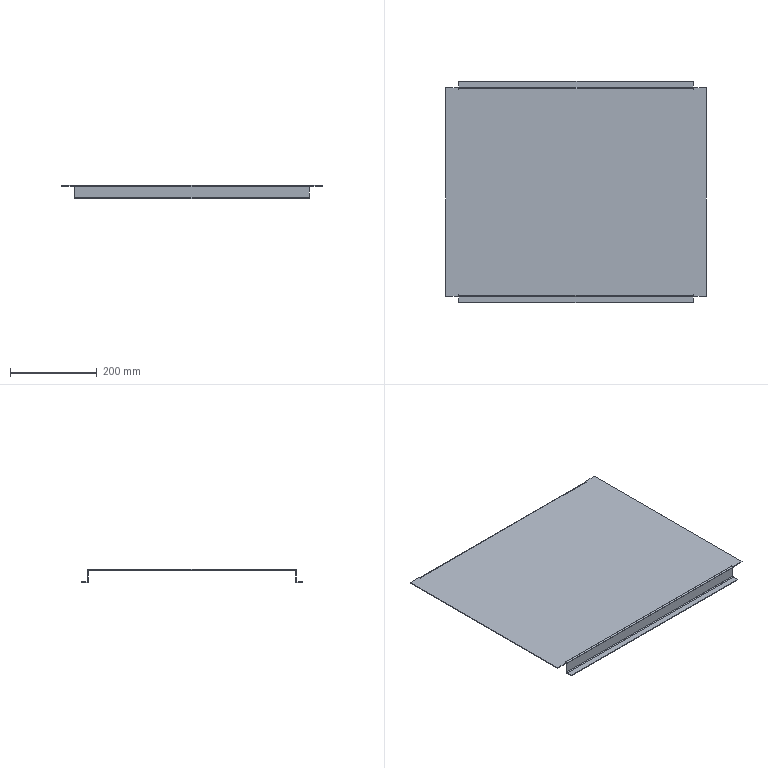Part | SolidWorks | features EdgeFlange 2, FlatPattern 1, SMBaseFlange 1, SheetMetal 1 | 1 solid | 54 faces | box 600 x 510 x 30 mm | volume 499324 mm3 | plane 46 | cylinder 8 | commonest cylinder face diameters 3 x4 6 x4
STEP:
#1=CARTESIAN_POINT('',(-270.,240.,-3.));
#2=VERTEX_POINT('',#1);
#3=CARTESIAN_POINT('',(-270.,240.,-27.));
#4=VERTEX_POINT('',#3);
#5=CARTESIAN_POINT('',(-270.,240.,-1.5));
#6=DIRECTION('',(0.,0.,-1.));
#7=VECTOR('',#6,1000.);
#8=LINE('',#5,#7);
#9=EDGE_CURVE('',#2,#4,#8,.T.);
#10=ORIENTED_EDGE('',*,*,#9,.T.);
#11=CARTESIAN_POINT('',(-270.,238.5,-27.));
#12=VERTEX_POINT('',#11);
#13=CARTESIAN_POINT('',(-270.,240.,-27.));
#14=DIRECTION('',(0.,-1.,0.));
#15=VECTOR('',#14,1000.);
#16=LINE('',#13,#15);
#17=EDGE_CURVE('',#4,#12,#16,.T.);
#18=ORIENTED_EDGE('',*,*,#17,.T.);
#19=CARTESIAN_POINT('',(-270.,238.5,-3.));
#20=VERTEX_POINT('',#19);
#21=CARTESIAN_POINT('',(-270.,238.5,0.));
#22=DIRECTION('',(0.,0.,-1.));
#23=VECTOR('',#22,1000.);
#24=LINE('',#21,#23);
#25=EDGE_CURVE('',#20,#12,#24,.T.);
#26=ORIENTED_EDGE('',*,*,#25,.F.);
#27=CARTESIAN_POINT('',(-270.,240.,-3.));
#28=DIRECTION('',(0.,1.,0.));
#29=VECTOR('',#28,1000.);
#30=LINE('',#27,#29);
#31=EDGE_CURVE('',#20,#2,#30,.T.);
#32=ORIENTED_EDGE('',*,*,#31,.T.);
#33=EDGE_LOOP('',(#10,#18,#26,#32));
#34=FACE_OUTER_BOUND('',#33,.T.);
#35=CARTESIAN_POINT('',(-270.,240.,-1.5));
#36=DIRECTION('',(-1.,0.,0.));
#37=DIRECTION('',(0.,0.,1.));
#38=AXIS2_PLACEMENT_3D('',#35,#36,#37);
#39=PLANE('',#38);
#40=ADVANCED_FACE('',(#34),#39,.T.);
#41=CARTESIAN_POINT('',(270.,240.,-27.));
#42=VERTEX_POINT('',#41);
#43=CARTESIAN_POINT('',(-270.,240.,-27.));
#44=DIRECTION('',(1.,0.,0.));
#45=VECTOR('',#44,1000.);
#46=LINE('',#43,#45);
#47=EDGE_CURVE('',#4,#42,#46,.T.);
#48=ORIENTED_EDGE('',*,*,#47,.F.);
#49=ORIENTED_EDGE('',*,*,#9,.F.);
#50=CARTESIAN_POINT('',(270.,240.,-3.));
#51=VERTEX_POINT('',#50);
#52=CARTESIAN_POINT('',(-270.,240.,-3.));
#53=DIRECTION('',(-1.,0.,0.));
#54=VECTOR('',#53,1000.);
#55=LINE('',#52,#54);
#56=EDGE_CURVE('',#51,#2,#55,.T.);
#57=ORIENTED_EDGE('',*,*,#56,.F.);
#58=CARTESIAN_POINT('',(270.,240.,-30.));
#59=DIRECTION('',(0.,0.,1.));
#60=VECTOR('',#59,1000.);
#61=LINE('',#58,#60);
#62=EDGE_CURVE('',#42,#51,#61,.T.);
#63=ORIENTED_EDGE('',*,*,#62,.F.);
#64=EDGE_LOOP('',(#48,#49,#57,#63));
#65=FACE_OUTER_BOUND('',#64,.T.);
#66=CARTESIAN_POINT('',(0.,240.,0.));
#67=DIRECTION('',(0.,-1.,0.));
#68=DIRECTION('',(0.,0.,-1.));
#69=AXIS2_PLACEMENT_3D('',#66,#67,#68);
#70=PLANE('',#69);
#71=ADVANCED_FACE('',(#65),#70,.F.);
#72=ORIENTED_EDGE('',*,*,#25,.T.);
#73=CARTESIAN_POINT('',(270.,238.5,-27.));
#74=VERTEX_POINT('',#73);
#75=CARTESIAN_POINT('',(-270.,238.5,-27.));
#76=DIRECTION('',(1.,0.,0.));
#77=VECTOR('',#76,1000.);
#78=LINE('',#75,#77);
#79=EDGE_CURVE('',#12,#74,#78,.T.);
#80=ORIENTED_EDGE('',*,*,#79,.T.);
#81=CARTESIAN_POINT('',(270.,238.5,-3.));
#82=VERTEX_POINT('',#81);
#83=CARTESIAN_POINT('',(270.,238.5,0.));
#84=DIRECTION('',(0.,0.,1.));
#85=VECTOR('',#84,1000.);
#86=LINE('',#83,#85);
#87=EDGE_CURVE('',#74,#82,#86,.T.);
#88=ORIENTED_EDGE('',*,*,#87,.T.);
#89=CARTESIAN_POINT('',(-270.,238.5,-3.));
#90=DIRECTION('',(1.,0.,0.));
#91=VECTOR('',#90,1000.);
#92=LINE('',#89,#91);
#93=EDGE_CURVE('',#20,#82,#92,.T.);
#94=ORIENTED_EDGE('',*,*,#93,.F.);
#95=EDGE_LOOP('',(#72,#80,#88,#94));
#96=FACE_OUTER_BOUND('',#95,.T.);
#97=CARTESIAN_POINT('',(0.,238.5,0.));
#98=DIRECTION('',(0.,-1.,0.));
#99=DIRECTION('',(0.,0.,-1.));
#100=AXIS2_PLACEMENT_3D('',#97,#98,#99);
#101=PLANE('',#100);
#102=ADVANCED_FACE('',(#96),#101,.T.);
#103=CARTESIAN_POINT('',(270.,-240.,-3.));
#104=VERTEX_POINT('',#103);
#105=CARTESIAN_POINT('',(270.,-240.,-27.));
#106=VERTEX_POINT('',#105);
#107=CARTESIAN_POINT('',(270.,-240.,-30.));
#108=DIRECTION('',(0.,0.,-1.));
#109=VECTOR('',#108,1000.);
#110=LINE('',#107,#109);
#111=EDGE_CURVE('',#104,#106,#110,.T.);
#112=ORIENTED_EDGE('',*,*,#111,.T.);
#113=CARTESIAN_POINT('',(270.,-238.5,-27.));
#114=VERTEX_POINT('',#113);
#115=CARTESIAN_POINT('',(270.,-240.,-27.));
#116=DIRECTION('',(0.,1.,0.));
#117=VECTOR('',#116,1000.);
#118=LINE('',#115,#117);
#119=EDGE_CURVE('',#106,#114,#118,.T.);
#120=ORIENTED_EDGE('',*,*,#119,.T.);
#121=CARTESIAN_POINT('',(270.,-238.5,-3.));
#122=VERTEX_POINT('',#121);
#123=CARTESIAN_POINT('',(270.,-238.5,0.));
#124=DIRECTION('',(0.,0.,-1.));
#125=VECTOR('',#124,1000.);
#126=LINE('',#123,#125);
#127=EDGE_CURVE('',#122,#114,#126,.T.);
#128=ORIENTED_EDGE('',*,*,#127,.F.);
#129=CARTESIAN_POINT('',(270.,-240.,-3.));
#130=DIRECTION('',(0.,-1.,0.));
#131=VECTOR('',#130,1000.);
#132=LINE('',#129,#131);
#133=EDGE_CURVE('',#122,#104,#132,.T.);
#134=ORIENTED_EDGE('',*,*,#133,.T.);
#135=EDGE_LOOP('',(#112,#120,#128,#134));
#136=FACE_OUTER_BOUND('',#135,.T.);
#137=CARTESIAN_POINT('',(270.,-240.,-30.));
#138=DIRECTION('',(1.,0.,0.));
#139=DIRECTION('',(0.,0.,-1.));
#140=AXIS2_PLACEMENT_3D('',#137,#138,#139);
#141=PLANE('',#140);
#142=ADVANCED_FACE('',(#136),#141,.T.);
#143=CARTESIAN_POINT('',(-270.,-240.,-27.));
#144=VERTEX_POINT('',#143);
#145=CARTESIAN_POINT('',(-270.,-240.,-3.));
#146=VERTEX_POINT('',#145);
#147=CARTESIAN_POINT('',(-270.,-240.,-1.5));
#148=DIRECTION('',(0.,0.,1.));
#149=VECTOR('',#148,1000.);
#150=LINE('',#147,#149);
#151=EDGE_CURVE('',#144,#146,#150,.T.);
#152=ORIENTED_EDGE('',*,*,#151,.F.);
#153=CARTESIAN_POINT('',(270.,-240.,-27.));
#154=DIRECTION('',(-1.,0.,0.));
#155=VECTOR('',#154,1000.);
#156=LINE('',#153,#155);
#157=EDGE_CURVE('',#106,#144,#156,.T.);
#158=ORIENTED_EDGE('',*,*,#157,.F.);
#159=ORIENTED_EDGE('',*,*,#111,.F.);
#160=CARTESIAN_POINT('',(0.,-240.,-3.));
#161=DIRECTION('',(-1.,0.,0.));
#162=VECTOR('',#161,1000.);
#163=LINE('',#160,#162);
#164=EDGE_CURVE('',#104,#146,#163,.T.);
#165=ORIENTED_EDGE('',*,*,#164,.T.);
#166=EDGE_LOOP('',(#152,#158,#159,#165));
#167=FACE_OUTER_BOUND('',#166,.T.);
#168=CARTESIAN_POINT('',(0.,-240.,0.));
#169=DIRECTION('',(0.,-1.,0.));
#170=DIRECTION('',(0.,0.,-1.));
#171=AXIS2_PLACEMENT_3D('',#168,#169,#170);
#172=PLANE('',#171);
#173=ADVANCED_FACE('',(#167),#172,.T.);
#174=CARTESIAN_POINT('',(-270.,-238.5,-27.));
#175=VERTEX_POINT('',#174);
#176=CARTESIAN_POINT('',(270.,-238.5,-27.));
#177=DIRECTION('',(-1.,0.,0.));
#178=VECTOR('',#177,1000.);
#179=LINE('',#176,#178);
#180=EDGE_CURVE('',#114,#175,#179,.T.);
#181=ORIENTED_EDGE('',*,*,#180,.T.);
#182=CARTESIAN_POINT('',(-270.,-238.5,-3.));
#183=VERTEX_POINT('',#182);
#184=CARTESIAN_POINT('',(-270.,-238.5,0.));
#185=DIRECTION('',(0.,0.,1.));
#186=VECTOR('',#185,1000.);
#187=LINE('',#184,#186);
#188=EDGE_CURVE('',#175,#183,#187,.T.);
#189=ORIENTED_EDGE('',*,*,#188,.T.);
#190=CARTESIAN_POINT('',(270.,-238.5,-3.));
#191=DIRECTION('',(-1.,0.,0.));
#192=VECTOR('',#191,1000.);
#193=LINE('',#190,#192);
#194=EDGE_CURVE('',#122,#183,#193,.T.);
#195=ORIENTED_EDGE('',*,*,#194,.F.);
#196=ORIENTED_EDGE('',*,*,#127,.T.);
#197=EDGE_LOOP('',(#181,#189,#195,#196));
#198=FACE_OUTER_BOUND('',#197,.T.);
#199=CARTESIAN_POINT('',(0.,-238.5,0.));
#200=DIRECTION('',(0.,-1.,0.));
#201=DIRECTION('',(0.,0.,-1.));
#202=AXIS2_PLACEMENT_3D('',#199,#200,#201);
#203=PLANE('',#202);
#204=ADVANCED_FACE('',(#198),#203,.F.);
#205=CARTESIAN_POINT('',(270.75,240.,-1.5));
#206=VERTEX_POINT('',#205);
#207=CARTESIAN_POINT('',(270.75,236.25,-1.5));
#208=VERTEX_POINT('',#207);
#209=CARTESIAN_POINT('',(270.75,240.,-1.5));
#210=DIRECTION('',(0.,-1.,0.));
#211=VECTOR('',#210,1000.);
#212=LINE('',#209,#211);
#213=EDGE_CURVE('',#206,#208,#212,.T.);
#214=ORIENTED_EDGE('',*,*,#213,.F.);
#215=CARTESIAN_POINT('',(300.,240.,-1.5));
#216=VERTEX_POINT('',#215);
#217=CARTESIAN_POINT('',(-300.,240.,-1.5));
#218=DIRECTION('',(-1.,0.,0.));
#219=VECTOR('',#218,1000.);
#220=LINE('',#217,#219);
#221=EDGE_CURVE('',#216,#206,#220,.T.);
#222=ORIENTED_EDGE('',*,*,#221,.F.);
#223=CARTESIAN_POINT('',(300.,-240.,-1.5));
#224=VERTEX_POINT('',#223);
#225=CARTESIAN_POINT('',(300.,240.,-1.5));
#226=DIRECTION('',(0.,1.,0.));
#227=VECTOR('',#226,1000.);
#228=LINE('',#225,#227);
#229=EDGE_CURVE('',#224,#216,#228,.T.);
#230=ORIENTED_EDGE('',*,*,#229,.F.);
#231=CARTESIAN_POINT('',(270.75,-240.,-1.5));
#232=VERTEX_POINT('',#231);
#233=CARTESIAN_POINT('',(-300.,-240.,-1.5));
#234=DIRECTION('',(1.,0.,0.));
#235=VECTOR('',#234,1000.);
#236=LINE('',#233,#235);
#237=EDGE_CURVE('',#232,#224,#236,.T.);
#238=ORIENTED_EDGE('',*,*,#237,.F.);
#239=CARTESIAN_POINT('',(270.75,-236.25,-1.5));
#240=VERTEX_POINT('',#239);
#241=CARTESIAN_POINT('',(270.75,-236.25,-1.5));
#242=DIRECTION('',(0.,-1.,0.));
#243=VECTOR('',#242,1000.);
#244=LINE('',#241,#243);
#245=EDGE_CURVE('',#240,#232,#244,.T.);
#246=ORIENTED_EDGE('',*,*,#245,.F.);
#247=CARTESIAN_POINT('',(270.,-236.25,-1.5));
#248=VERTEX_POINT('',#247);
#249=CARTESIAN_POINT('',(270.,-236.25,-1.5));
#250=DIRECTION('',(1.,0.,0.));
#251=VECTOR('',#250,1000.);
#252=LINE('',#249,#251);
#253=EDGE_CURVE('',#248,#240,#252,.T.);
#254=ORIENTED_EDGE('',*,*,#253,.F.);
#255=CARTESIAN_POINT('',(270.,-237.,-1.5));
#256=VERTEX_POINT('',#255);
#257=CARTESIAN_POINT('',(270.,-237.,-1.5));
#258=DIRECTION('',(0.,1.,0.));
#259=VECTOR('',#258,1000.);
#260=LINE('',#257,#259);
#261=EDGE_CURVE('',#256,#248,#260,.T.);
#262=ORIENTED_EDGE('',*,*,#261,.F.);
#263=CARTESIAN_POINT('',(-270.,-237.,-1.5));
#264=VERTEX_POINT('',#263);
#265=CARTESIAN_POINT('',(-270.,-237.,-1.5));
#266=DIRECTION('',(1.,0.,0.));
#267=VECTOR('',#266,1000.);
#268=LINE('',#265,#267);
#269=EDGE_CURVE('',#264,#256,#268,.T.);
#270=ORIENTED_EDGE('',*,*,#269,.F.);
#271=CARTESIAN_POINT('',(-270.,-236.25,-1.5));
#272=VERTEX_POINT('',#271);
#273=CARTESIAN_POINT('',(-270.,-236.25,-1.5));
#274=DIRECTION('',(0.,-1.,0.));
#275=VECTOR('',#274,1000.);
#276=LINE('',#273,#275);
#277=EDGE_CURVE('',#272,#264,#276,.T.);
#278=ORIENTED_EDGE('',*,*,#277,.F.);
#279=CARTESIAN_POINT('',(-270.75,-236.25,-1.5));
#280=VERTEX_POINT('',#279);
#281=CARTESIAN_POINT('',(-270.75,-236.25,-1.5));
#282=DIRECTION('',(1.,0.,0.));
#283=VECTOR('',#282,1000.);
#284=LINE('',#281,#283);
#285=EDGE_CURVE('',#280,#272,#284,.T.);
#286=ORIENTED_EDGE('',*,*,#285,.F.);
#287=CARTESIAN_POINT('',(-270.75,-240.,-1.5));
#288=VERTEX_POINT('',#287);
#289=CARTESIAN_POINT('',(-270.75,-240.,-1.5));
#290=DIRECTION('',(0.,1.,0.));
#291=VECTOR('',#290,1000.);
#292=LINE('',#289,#291);
#293=EDGE_CURVE('',#288,#280,#292,.T.);
#294=ORIENTED_EDGE('',*,*,#293,.F.);
#295=CARTESIAN_POINT('',(-300.,-240.,-1.5));
#296=VERTEX_POINT('',#295);
#297=CARTESIAN_POINT('',(-300.,-240.,-1.5));
#298=DIRECTION('',(1.,0.,0.));
#299=VECTOR('',#298,1000.);
#300=LINE('',#297,#299);
#301=EDGE_CURVE('',#296,#288,#300,.T.);
#302=ORIENTED_EDGE('',*,*,#301,.F.);
#303=CARTESIAN_POINT('',(-300.,240.,-1.5));
#304=VERTEX_POINT('',#303);
#305=CARTESIAN_POINT('',(-300.,240.,-1.5));
#306=DIRECTION('',(0.,-1.,0.));
#307=VECTOR('',#306,1000.);
#308=LINE('',#305,#307);
#309=EDGE_CURVE('',#304,#296,#308,.T.);
#310=ORIENTED_EDGE('',*,*,#309,.F.);
#311=CARTESIAN_POINT('',(-270.75,240.,-1.5));
#312=VERTEX_POINT('',#311);
#313=CARTESIAN_POINT('',(-300.,240.,-1.5));
#314=DIRECTION('',(-1.,0.,0.));
#315=VECTOR('',#314,1000.);
#316=LINE('',#313,#315);
#317=EDGE_CURVE('',#312,#304,#316,.T.);
#318=ORIENTED_EDGE('',*,*,#317,.F.);
#319=CARTESIAN_POINT('',(-270.75,236.25,-1.5));
#320=VERTEX_POINT('',#319);
#321=CARTESIAN_POINT('',(-270.75,236.25,-1.5));
#322=DIRECTION('',(0.,1.,0.));
#323=VECTOR('',#322,1000.);
#324=LINE('',#321,#323);
#325=EDGE_CURVE('',#320,#312,#324,.T.);
#326=ORIENTED_EDGE('',*,*,#325,.F.);
#327=CARTESIAN_POINT('',(-270.,236.25,-1.5));
#328=VERTEX_POINT('',#327);
#329=CARTESIAN_POINT('',(-270.,236.25,-1.5));
#330=DIRECTION('',(-1.,0.,0.));
#331=VECTOR('',#330,1000.);
#332=LINE('',#329,#331);
#333=EDGE_CURVE('',#328,#320,#332,.T.);
#334=ORIENTED_EDGE('',*,*,#333,.F.);
#335=CARTESIAN_POINT('',(-270.,237.,-1.5));
#336=VERTEX_POINT('',#335);
#337=CARTESIAN_POINT('',(-270.,237.,-1.5));
#338=DIRECTION('',(0.,-1.,0.));
#339=VECTOR('',#338,1000.);
#340=LINE('',#337,#339);
#341=EDGE_CURVE('',#336,#328,#340,.T.);
#342=ORIENTED_EDGE('',*,*,#341,.F.);
#343=CARTESIAN_POINT('',(270.,237.,-1.5));
#344=VERTEX_POINT('',#343);
#345=CARTESIAN_POINT('',(270.,237.,-1.5));
#346=DIRECTION('',(-1.,0.,0.));
#347=VECTOR('',#346,1000.);
#348=LINE('',#345,#347);
#349=EDGE_CURVE('',#344,#336,#348,.T.);
#350=ORIENTED_EDGE('',*,*,#349,.F.);
#351=CARTESIAN_POINT('',(270.,236.25,-1.5));
#352=VERTEX_POINT('',#351);
#353=CARTESIAN_POINT('',(270.,236.25,-1.5));
#354=DIRECTION('',(0.,1.,0.));
#355=VECTOR('',#354,1000.);
#356=LINE('',#353,#355);
#357=EDGE_CURVE('',#352,#344,#356,.T.);
#358=ORIENTED_EDGE('',*,*,#357,.F.);
#359=CARTESIAN_POINT('',(270.75,236.25,-1.5));
#360=DIRECTION('',(-1.,0.,0.));
#361=VECTOR('',#360,1000.);
#362=LINE('',#359,#361);
#363=EDGE_CURVE('',#208,#352,#362,.T.);
#364=ORIENTED_EDGE('',*,*,#363,.F.);
#365=EDGE_LOOP('',(#214,#222,#230,#238,#246,#254,#262,#270,#278,#286,#294,#302,#310,#318,#326,#334,#342,#350,#358,#364));
#366=FACE_OUTER_BOUND('',#365,.T.);
#367=CARTESIAN_POINT('',(0.,0.,-1.5));
#368=DIRECTION('',(0.,0.,1.));
#369=DIRECTION('',(1.,0.,0.));
#370=AXIS2_PLACEMENT_3D('',#367,#368,#369);
#371=PLANE('',#370);
#372=ADVANCED_FACE('',(#366),#371,.F.);
#373=CARTESIAN_POINT('',(300.,240.,0.));
#374=VERTEX_POINT('',#373);
#375=CARTESIAN_POINT('',(270.75,240.,0.));
#376=VERTEX_POINT('',#375);
#377=CARTESIAN_POINT('',(-300.,240.,0.));
#378=DIRECTION('',(-1.,0.,0.));
#379=VECTOR('',#378,1000.);
#380=LINE('',#377,#379);
#381=EDGE_CURVE('',#374,#376,#380,.T.);
#382=ORIENTED_EDGE('',*,*,#381,.T.);
#383=CARTESIAN_POINT('',(270.75,236.25,0.));
#384=VERTEX_POINT('',#383);
#385=CARTESIAN_POINT('',(270.75,0.,0.));
#386=DIRECTION('',(0.,-1.,0.));
#387=VECTOR('',#386,1000.);
#388=LINE('',#385,#387);
#389=EDGE_CURVE('',#376,#384,#388,.T.);
#390=ORIENTED_EDGE('',*,*,#389,.T.);
#391=CARTESIAN_POINT('',(270.,236.25,0.));
#392=VERTEX_POINT('',#391);
#393=CARTESIAN_POINT('',(0.,236.25,0.));
#394=DIRECTION('',(-1.,0.,0.));
#395=VECTOR('',#394,1000.);
#396=LINE('',#393,#395);
#397=EDGE_CURVE('',#384,#392,#396,.T.);
#398=ORIENTED_EDGE('',*,*,#397,.T.);
#399=CARTESIAN_POINT('',(270.,237.,0.));
#400=VERTEX_POINT('',#399);
#401=CARTESIAN_POINT('',(270.,0.,0.));
#402=DIRECTION('',(0.,1.,0.));
#403=VECTOR('',#402,1000.);
#404=LINE('',#401,#403);
#405=EDGE_CURVE('',#392,#400,#404,.T.);
#406=ORIENTED_EDGE('',*,*,#405,.T.);
#407=CARTESIAN_POINT('',(-270.,237.,0.));
#408=VERTEX_POINT('',#407);
#409=CARTESIAN_POINT('',(270.,237.,0.));
#410=DIRECTION('',(-1.,0.,0.));
#411=VECTOR('',#410,1000.);
#412=LINE('',#409,#411);
#413=EDGE_CURVE('',#400,#408,#412,.T.);
#414=ORIENTED_EDGE('',*,*,#413,.T.);
#415=CARTESIAN_POINT('',(-270.,236.25,0.));
#416=VERTEX_POINT('',#415);
#417=CARTESIAN_POINT('',(-270.,0.,0.));
#418=DIRECTION('',(0.,-1.,0.));
#419=VECTOR('',#418,1000.);
#420=LINE('',#417,#419);
#421=EDGE_CURVE('',#408,#416,#420,.T.);
#422=ORIENTED_EDGE('',*,*,#421,.T.);
#423=CARTESIAN_POINT('',(-270.75,236.25,0.));
#424=VERTEX_POINT('',#423);
#425=CARTESIAN_POINT('',(0.,236.25,0.));
#426=DIRECTION('',(-1.,0.,0.));
#427=VECTOR('',#426,1000.);
#428=LINE('',#425,#427);
#429=EDGE_CURVE('',#416,#424,#428,.T.);
#430=ORIENTED_EDGE('',*,*,#429,.T.);
#431=CARTESIAN_POINT('',(-270.75,240.,0.));
#432=VERTEX_POINT('',#431);
#433=CARTESIAN_POINT('',(-270.75,0.,0.));
#434=DIRECTION('',(0.,1.,0.));
#435=VECTOR('',#434,1000.);
#436=LINE('',#433,#435);
#437=EDGE_CURVE('',#424,#432,#436,.T.);
#438=ORIENTED_EDGE('',*,*,#437,.T.);
#439=CARTESIAN_POINT('',(-300.,240.,0.));
#440=VERTEX_POINT('',#439);
#441=CARTESIAN_POINT('',(-300.,240.,0.));
#442=DIRECTION('',(-1.,0.,0.));
#443=VECTOR('',#442,1000.);
#444=LINE('',#441,#443);
#445=EDGE_CURVE('',#432,#440,#444,.T.);
#446=ORIENTED_EDGE('',*,*,#445,.T.);
#447=CARTESIAN_POINT('',(-300.,-240.,0.));
#448=VERTEX_POINT('',#447);
#449=CARTESIAN_POINT('',(-300.,240.,0.));
#450=DIRECTION('',(0.,-1.,0.));
#451=VECTOR('',#450,1000.);
#452=LINE('',#449,#451);
#453=EDGE_CURVE('',#440,#448,#452,.T.);
#454=ORIENTED_EDGE('',*,*,#453,.T.);
#455=CARTESIAN_POINT('',(-270.75,-240.,0.));
#456=VERTEX_POINT('',#455);
#457=CARTESIAN_POINT('',(-300.,-240.,0.));
#458=DIRECTION('',(1.,0.,0.));
#459=VECTOR('',#458,1000.);
#460=LINE('',#457,#459);
#461=EDGE_CURVE('',#448,#456,#460,.T.);
#462=ORIENTED_EDGE('',*,*,#461,.T.);
#463=CARTESIAN_POINT('',(-270.75,-236.25,0.));
#464=VERTEX_POINT('',#463);
#465=CARTESIAN_POINT('',(-270.75,0.,0.));
#466=DIRECTION('',(0.,1.,0.));
#467=VECTOR('',#466,1000.);
#468=LINE('',#465,#467);
#469=EDGE_CURVE('',#456,#464,#468,.T.);
#470=ORIENTED_EDGE('',*,*,#469,.T.);
#471=CARTESIAN_POINT('',(-270.,-236.25,0.));
#472=VERTEX_POINT('',#471);
#473=CARTESIAN_POINT('',(0.,-236.25,0.));
#474=DIRECTION('',(1.,0.,0.));
#475=VECTOR('',#474,1000.);
#476=LINE('',#473,#475);
#477=EDGE_CURVE('',#464,#472,#476,.T.);
#478=ORIENTED_EDGE('',*,*,#477,.T.);
#479=CARTESIAN_POINT('',(-270.,-237.,0.));
#480=VERTEX_POINT('',#479);
#481=CARTESIAN_POINT('',(-270.,0.,0.));
#482=DIRECTION('',(0.,-1.,0.));
#483=VECTOR('',#482,1000.);
#484=LINE('',#481,#483);
#485=EDGE_CURVE('',#472,#480,#484,.T.);
#486=ORIENTED_EDGE('',*,*,#485,.T.);
#487=CARTESIAN_POINT('',(270.,-237.,0.));
#488=VERTEX_POINT('',#487);
#489=CARTESIAN_POINT('',(-270.,-237.,0.));
#490=DIRECTION('',(1.,0.,0.));
#491=VECTOR('',#490,1000.);
#492=LINE('',#489,#491);
#493=EDGE_CURVE('',#480,#488,#492,.T.);
#494=ORIENTED_EDGE('',*,*,#493,.T.);
#495=CARTESIAN_POINT('',(270.,-236.25,0.));
#496=VERTEX_POINT('',#495);
#497=CARTESIAN_POINT('',(270.,0.,0.));
#498=DIRECTION('',(0.,1.,0.));
#499=VECTOR('',#498,1000.);
#500=LINE('',#497,#499);
#501=EDGE_CURVE('',#488,#496,#500,.T.);
#502=ORIENTED_EDGE('',*,*,#501,.T.);
#503=CARTESIAN_POINT('',(270.75,-236.25,0.));
#504=VERTEX_POINT('',#503);
#505=CARTESIAN_POINT('',(0.,-236.25,0.));
#506=DIRECTION('',(1.,0.,0.));
#507=VECTOR('',#506,1000.);
#508=LINE('',#505,#507);
#509=EDGE_CURVE('',#496,#504,#508,.T.);
#510=ORIENTED_EDGE('',*,*,#509,.T.);
#511=CARTESIAN_POINT('',(270.75,-240.,0.));
#512=VERTEX_POINT('',#511);
#513=CARTESIAN_POINT('',(270.75,0.,0.));
#514=DIRECTION('',(0.,-1.,0.));
#515=VECTOR('',#514,1000.);
#516=LINE('',#513,#515);
#517=EDGE_CURVE('',#504,#512,#516,.T.);
#518=ORIENTED_EDGE('',*,*,#517,.T.);
#519=CARTESIAN_POINT('',(300.,-240.,0.));
#520=VERTEX_POINT('',#519);
#521=CARTESIAN_POINT('',(-300.,-240.,0.));
#522=DIRECTION('',(1.,0.,0.));
#523=VECTOR('',#522,1000.);
#524=LINE('',#521,#523);
#525=EDGE_CURVE('',#512,#520,#524,.T.);
#526=ORIENTED_EDGE('',*,*,#525,.T.);
#527=CARTESIAN_POINT('',(300.,240.,0.));
#528=DIRECTION('',(0.,1.,0.));
#529=VECTOR('',#528,1000.);
#530=LINE('',#527,#529);
#531=EDGE_CURVE('',#520,#374,#530,.T.);
#532=ORIENTED_EDGE('',*,*,#531,.T.);
#533=EDGE_LOOP('',(#382,#390,#398,#406,#414,#422,#430,#438,#446,#454,#462,#470,#478,#486,#494,#502,#510,#518,#526,#532));
#534=FACE_OUTER_BOUND('',#533,.T.);
#535=CARTESIAN_POINT('',(0.,0.,0.));
#536=DIRECTION('',(0.,0.,1.));
#537=DIRECTION('',(1.,0.,0.));
#538=AXIS2_PLACEMENT_3D('',#535,#536,#537);
#539=PLANE('',#538);
#540=ADVANCED_FACE('',(#534),#539,.T.);
#541=ORIENTED_EDGE('',*,*,#221,.T.);
#542=CARTESIAN_POINT('',(270.75,240.,-1.5));
#543=DIRECTION('',(0.,0.,1.));
#544=VECTOR('',#543,1000.);
#545=LINE('',#542,#544);
#546=EDGE_CURVE('',#206,#376,#545,.T.);
#547=ORIENTED_EDGE('',*,*,#546,.T.);
#548=ORIENTED_EDGE('',*,*,#381,.F.);
#549=CARTESIAN_POINT('',(300.,240.,-1.5));
#550=DIRECTION('',(0.,0.,1.));
#551=VECTOR('',#550,1000.);
#552=LINE('',#549,#551);
#553=EDGE_CURVE('',#216,#374,#552,.T.);
#554=ORIENTED_EDGE('',*,*,#553,.F.);
#555=EDGE_LOOP('',(#541,#547,#548,#554));
#556=FACE_OUTER_BOUND('',#555,.T.);
#557=CARTESIAN_POINT('',(-300.,240.,-1.5));
#558=DIRECTION('',(0.,1.,0.));
#559=DIRECTION('',(0.,0.,1.));
#560=AXIS2_PLACEMENT_3D('',#557,#558,#559);
#561=PLANE('',#560);
#562=ADVANCED_FACE('',(#556),#561,.T.);
#563=ORIENTED_EDGE('',*,*,#445,.F.);
#564=CARTESIAN_POINT('',(-270.75,240.,-1.5));
#565=DIRECTION('',(0.,0.,1.));
#566=VECTOR('',#565,1000.);
#567=LINE('',#564,#566);
#568=EDGE_CURVE('',#312,#432,#567,.T.);
#569=ORIENTED_EDGE('',*,*,#568,.F.);
#570=ORIENTED_EDGE('',*,*,#317,.T.);
#571=CARTESIAN_POINT('',(-300.,240.,-1.5));
#572=DIRECTION('',(0.,0.,1.));
#573=VECTOR('',#572,1000.);
#574=LINE('',#571,#573);
#575=EDGE_CURVE('',#304,#440,#574,.T.);
#576=ORIENTED_EDGE('',*,*,#575,.T.);
#577=EDGE_LOOP('',(#563,#569,#570,#576));
#578=FACE_OUTER_BOUND('',#577,.T.);
#579=CARTESIAN_POINT('',(-300.,240.,-1.5));
#580=DIRECTION('',(0.,1.,0.));
#581=DIRECTION('',(0.,0.,1.));
#582=AXIS2_PLACEMENT_3D('',#579,#580,#581);
#583=PLANE('',#582);
#584=ADVANCED_FACE('',(#578),#583,.T.);
#585=ORIENTED_EDGE('',*,*,#301,.T.);
#586=CARTESIAN_POINT('',(-270.75,-240.,-1.5));
#587=DIRECTION('',(0.,0.,1.));
#588=VECTOR('',#587,1000.);
#589=LINE('',#586,#588);
#590=EDGE_CURVE('',#288,#456,#589,.T.);
#591=ORIENTED_EDGE('',*,*,#590,.T.);
#592=ORIENTED_EDGE('',*,*,#461,.F.);
#593=CARTESIAN_POINT('',(-300.,-240.,-1.5));
#594=DIRECTION('',(0.,0.,1.));
#595=VECTOR('',#594,1000.);
#596=LINE('',#593,#595);
#597=EDGE_CURVE('',#296,#448,#596,.T.);
#598=ORIENTED_EDGE('',*,*,#597,.F.);
#599=EDGE_LOOP('',(#585,#591,#592,#598));
#600=FACE_OUTER_BOUND('',#599,.T.);
#601=CARTESIAN_POINT('',(-300.,-240.,-1.5));
#602=DIRECTION('',(0.,-1.,0.));
#603=DIRECTION('',(0.,0.,-1.));
#604=AXIS2_PLACEMENT_3D('',#601,#602,#603);
#605=PLANE('',#604);
#606=ADVANCED_FACE('',(#600),#605,.T.);
#607=ORIENTED_EDGE('',*,*,#525,.F.);
#608=CARTESIAN_POINT('',(270.75,-240.,-1.5));
#609=DIRECTION('',(0.,0.,1.));
#610=VECTOR('',#609,1000.);
#611=LINE('',#608,#610);
#612=EDGE_CURVE('',#232,#512,#611,.T.);
#613=ORIENTED_EDGE('',*,*,#612,.F.);
#614=ORIENTED_EDGE('',*,*,#237,.T.);
#615=CARTESIAN_POINT('',(300.,-240.,-1.5));
#616=DIRECTION('',(0.,0.,1.));
#617=VECTOR('',#616,1000.);
#618=LINE('',#615,#617);
#619=EDGE_CURVE('',#224,#520,#618,.T.);
#620=ORIENTED_EDGE('',*,*,#619,.T.);
#621=EDGE_LOOP('',(#607,#613,#614,#620));
#622=FACE_OUTER_BOUND('',#621,.T.);
#623=CARTESIAN_POINT('',(-300.,-240.,-1.5));
#624=DIRECTION('',(0.,-1.,0.));
#625=DIRECTION('',(0.,0.,-1.));
#626=AXIS2_PLACEMENT_3D('',#623,#624,#625);
#627=PLANE('',#626);
#628=ADVANCED_FACE('',(#622),#627,.T.);
#629=ORIENTED_EDGE('',*,*,#531,.F.);
#630=ORIENTED_EDGE('',*,*,#619,.F.);
#631=ORIENTED_EDGE('',*,*,#229,.T.);
#632=ORIENTED_EDGE('',*,*,#553,.T.);
#633=EDGE_LOOP('',(#629,#630,#631,#632));
#634=FACE_OUTER_BOUND('',#633,.T.);
#635=CARTESIAN_POINT('',(300.,240.,-1.5));
#636=DIRECTION('',(1.,0.,0.));
#637=DIRECTION('',(0.,1.,0.));
#638=AXIS2_PLACEMENT_3D('',#635,#636,#637);
#639=PLANE('',#638);
#640=ADVANCED_FACE('',(#634),#639,.T.);
#641=ORIENTED_EDGE('',*,*,#453,.F.);
#642=ORIENTED_EDGE('',*,*,#575,.F.);
#643=ORIENTED_EDGE('',*,*,#309,.T.);
#644=ORIENTED_EDGE('',*,*,#597,.T.);
#645=EDGE_LOOP('',(#641,#642,#643,#644));
#646=FACE_OUTER_BOUND('',#645,.T.);
#647=CARTESIAN_POINT('',(-300.,240.,-1.5));
#648=DIRECTION('',(-1.,0.,0.));
#649=DIRECTION('',(0.,-1.,0.));
#650=AXIS2_PLACEMENT_3D('',#647,#648,#649);
#651=PLANE('',#650);
#652=ADVANCED_FACE('',(#646),#651,.T.);
#653=ORIENTED_EDGE('',*,*,#469,.F.);
#654=ORIENTED_EDGE('',*,*,#590,.F.);
#655=ORIENTED_EDGE('',*,*,#293,.T.);
#656=CARTESIAN_POINT('',(-270.75,-236.25,-1.5));
#657=DIRECTION('',(0.,0.,1.));
#658=VECTOR('',#657,1000.);
#659=LINE('',#656,#658);
#660=EDGE_CURVE('',#280,#464,#659,.T.);
#661=ORIENTED_EDGE('',*,*,#660,.T.);
#662=EDGE_LOOP('',(#653,#654,#655,#661));
#663=FACE_OUTER_BOUND('',#662,.T.);
#664=CARTESIAN_POINT('',(-270.75,-240.,-1.5));
#665=DIRECTION('',(1.,0.,0.));
#666=DIRECTION('',(0.,0.,-1.));
#667=AXIS2_PLACEMENT_3D('',#664,#665,#666);
#668=PLANE('',#667);
#669=ADVANCED_FACE('',(#663),#668,.T.);
#670=ORIENTED_EDGE('',*,*,#477,.F.);
#671=ORIENTED_EDGE('',*,*,#660,.F.);
#672=ORIENTED_EDGE('',*,*,#285,.T.);
#673=CARTESIAN_POINT('',(-270.,-236.25,-1.5));
#674=DIRECTION('',(0.,0.,1.));
#675=VECTOR('',#674,1000.);
#676=LINE('',#673,#675);
#677=EDGE_CURVE('',#272,#472,#676,.T.);
#678=ORIENTED_EDGE('',*,*,#677,.T.);
#679=EDGE_LOOP('',(#670,#671,#672,#678));
#680=FACE_OUTER_BOUND('',#679,.T.);
#681=CARTESIAN_POINT('',(-270.75,-236.25,-1.5));
#682=DIRECTION('',(0.,-1.,0.));
#683=DIRECTION('',(0.,0.,-1.));
#684=AXIS2_PLACEMENT_3D('',#681,#682,#683);
#685=PLANE('',#684);
#686=ADVANCED_FACE('',(#680),#685,.T.);
#687=ORIENTED_EDGE('',*,*,#485,.F.);
#688=ORIENTED_EDGE('',*,*,#677,.F.);
#689=ORIENTED_EDGE('',*,*,#277,.T.);
#690=CARTESIAN_POINT('',(-270.,-237.,-1.5));
#691=DIRECTION('',(0.,0.,1.));
#692=VECTOR('',#691,1000.);
#693=LINE('',#690,#692);
#694=EDGE_CURVE('',#264,#480,#693,.T.);
#695=ORIENTED_EDGE('',*,*,#694,.T.);
#696=EDGE_LOOP('',(#687,#688,#689,#695));
#697=FACE_OUTER_BOUND('',#696,.T.);
#698=CARTESIAN_POINT('',(-270.,-236.25,-1.5));
#699=DIRECTION('',(-1.,0.,0.));
#700=DIRECTION('',(0.,0.,1.));
#701=AXIS2_PLACEMENT_3D('',#698,#699,#700);
#702=PLANE('',#701);
#703=ADVANCED_FACE('',(#697),#702,.T.);
#704=ORIENTED_EDGE('',*,*,#501,.F.);
#705=CARTESIAN_POINT('',(270.,-237.,-1.5));
#706=DIRECTION('',(0.,0.,1.));
#707=VECTOR('',#706,1000.);
#708=LINE('',#705,#707);
#709=EDGE_CURVE('',#256,#488,#708,.T.);
#710=ORIENTED_EDGE('',*,*,#709,.F.);
#711=ORIENTED_EDGE('',*,*,#261,.T.);
#712=CARTESIAN_POINT('',(270.,-236.25,-1.5));
#713=DIRECTION('',(0.,0.,1.));
#714=VECTOR('',#713,1000.);
#715=LINE('',#712,#714);
#716=EDGE_CURVE('',#248,#496,#715,.T.);
#717=ORIENTED_EDGE('',*,*,#716,.T.);
#718=EDGE_LOOP('',(#704,#710,#711,#717));
#719=FACE_OUTER_BOUND('',#718,.T.);
#720=CARTESIAN_POINT('',(270.,-237.,-1.5));
#721=DIRECTION('',(1.,0.,0.));
#722=DIRECTION('',(0.,0.,-1.));
#723=AXIS2_PLACEMENT_3D('',#720,#721,#722);
#724=PLANE('',#723);
#725=ADVANCED_FACE('',(#719),#724,.T.);
#726=ORIENTED_EDGE('',*,*,#509,.F.);
#727=ORIENTED_EDGE('',*,*,#716,.F.);
#728=ORIENTED_EDGE('',*,*,#253,.T.);
#729=CARTESIAN_POINT('',(270.75,-236.25,-1.5));
#730=DIRECTION('',(0.,0.,1.));
#731=VECTOR('',#730,1000.);
#732=LINE('',#729,#731);
#733=EDGE_CURVE('',#240,#504,#732,.T.);
#734=ORIENTED_EDGE('',*,*,#733,.T.);
#735=EDGE_LOOP('',(#726,#727,#728,#734));
#736=FACE_OUTER_BOUND('',#735,.T.);
#737=CARTESIAN_POINT('',(270.,-236.25,-1.5));
#738=DIRECTION('',(0.,-1.,0.));
#739=DIRECTION('',(0.,0.,-1.));
#740=AXIS2_PLACEMENT_3D('',#737,#738,#739);
#741=PLANE('',#740);
#742=ADVANCED_FACE('',(#736),#741,.T.);
#743=ORIENTED_EDGE('',*,*,#517,.F.);
#744=ORIENTED_EDGE('',*,*,#733,.F.);
#745=ORIENTED_EDGE('',*,*,#245,.T.);
#746=ORIENTED_EDGE('',*,*,#612,.T.);
#747=EDGE_LOOP('',(#743,#744,#745,#746));
#748=FACE_OUTER_BOUND('',#747,.T.);
#749=CARTESIAN_POINT('',(270.75,-236.25,-1.5));
#750=DIRECTION('',(-1.,0.,0.));
#751=DIRECTION('',(0.,-1.,0.));
#752=AXIS2_PLACEMENT_3D('',#749,#750,#751);
#753=PLANE('',#752);
#754=ADVANCED_FACE('',(#748),#753,.T.);
#755=ORIENTED_EDGE('',*,*,#389,.F.);
#756=ORIENTED_EDGE('',*,*,#546,.F.);
#757=ORIENTED_EDGE('',*,*,#213,.T.);
#758=CARTESIAN_POINT('',(270.75,236.25,-1.5));
#759=DIRECTION('',(0.,0.,1.));
#760=VECTOR('',#759,1000.);
#761=LINE('',#758,#760);
#762=EDGE_CURVE('',#208,#384,#761,.T.);
#763=ORIENTED_EDGE('',*,*,#762,.T.);
#764=EDGE_LOOP('',(#755,#756,#757,#763));
#765=FACE_OUTER_BOUND('',#764,.T.);
#766=CARTESIAN_POINT('',(270.75,240.,-1.5));
#767=DIRECTION('',(-1.,0.,0.));
#768=DIRECTION('',(0.,0.,1.));
#769=AXIS2_PLACEMENT_3D('',#766,#767,#768);
#770=PLANE('',#769);
#771=ADVANCED_FACE('',(#765),#770,.T.);
#772=ORIENTED_EDGE('',*,*,#397,.F.);
#773=ORIENTED_EDGE('',*,*,#762,.F.);
#774=ORIENTED_EDGE('',*,*,#363,.T.);
#775=CARTESIAN_POINT('',(270.,236.25,-1.5));
#776=DIRECTION('',(0.,0.,1.));
#777=VECTOR('',#776,1000.);
#778=LINE('',#775,#777);
#779=EDGE_CURVE('',#352,#392,#778,.T.);
#780=ORIENTED_EDGE('',*,*,#779,.T.);
#781=EDGE_LOOP('',(#772,#773,#774,#780));
#782=FACE_OUTER_BOUND('',#781,.T.);
#783=CARTESIAN_POINT('',(270.75,236.25,-1.5));
#784=DIRECTION('',(0.,1.,0.));
#785=DIRECTION('',(0.,0.,1.));
#786=AXIS2_PLACEMENT_3D('',#783,#784,#785);
#787=PLANE('',#786);
#788=ADVANCED_FACE('',(#782),#787,.T.);
#789=ORIENTED_EDGE('',*,*,#405,.F.);
#790=ORIENTED_EDGE('',*,*,#779,.F.);
#791=ORIENTED_EDGE('',*,*,#357,.T.);
#792=CARTESIAN_POINT('',(270.,237.,-1.5));
#793=DIRECTION('',(0.,0.,1.));
#794=VECTOR('',#793,1000.);
#795=LINE('',#792,#794);
#796=EDGE_CURVE('',#344,#400,#795,.T.);
#797=ORIENTED_EDGE('',*,*,#796,.T.);
#798=EDGE_LOOP('',(#789,#790,#791,#797));
#799=FACE_OUTER_BOUND('',#798,.T.);
#800=CARTESIAN_POINT('',(270.,236.25,-1.5));
#801=DIRECTION('',(1.,0.,0.));
#802=DIRECTION('',(0.,0.,-1.));
#803=AXIS2_PLACEMENT_3D('',#800,#801,#802);
#804=PLANE('',#803);
#805=ADVANCED_FACE('',(#799),#804,.T.);
#806=ORIENTED_EDGE('',*,*,#421,.F.);
#807=CARTESIAN_POINT('',(-270.,237.,-1.5));
#808=DIRECTION('',(0.,0.,1.));
#809=VECTOR('',#808,1000.);
#810=LINE('',#807,#809);
#811=EDGE_CURVE('',#336,#408,#810,.T.);
#812=ORIENTED_EDGE('',*,*,#811,.F.);
#813=ORIENTED_EDGE('',*,*,#341,.T.);
#814=CARTESIAN_POINT('',(-270.,236.25,-1.5));
#815=DIRECTION('',(0.,0.,1.));
#816=VECTOR('',#815,1000.);
#817=LINE('',#814,#816);
#818=EDGE_CURVE('',#328,#416,#817,.T.);
#819=ORIENTED_EDGE('',*,*,#818,.T.);
#820=EDGE_LOOP('',(#806,#812,#813,#819));
#821=FACE_OUTER_BOUND('',#820,.T.);
#822=CARTESIAN_POINT('',(-270.,237.,-1.5));
#823=DIRECTION('',(-1.,0.,0.));
#824=DIRECTION('',(0.,0.,1.));
#825=AXIS2_PLACEMENT_3D('',#822,#823,#824);
#826=PLANE('',#825);
#827=ADVANCED_FACE('',(#821),#826,.T.);
#828=ORIENTED_EDGE('',*,*,#429,.F.);
#829=ORIENTED_EDGE('',*,*,#818,.F.);
#830=ORIENTED_EDGE('',*,*,#333,.T.);
#831=CARTESIAN_POINT('',(-270.75,236.25,-1.5));
#832=DIRECTION('',(0.,0.,1.));
#833=VECTOR('',#832,1000.);
#834=LINE('',#831,#833);
#835=EDGE_CURVE('',#320,#424,#834,.T.);
#836=ORIENTED_EDGE('',*,*,#835,.T.);
#837=EDGE_LOOP('',(#828,#829,#830,#836));
#838=FACE_OUTER_BOUND('',#837,.T.);
#839=CARTESIAN_POINT('',(-270.,236.25,-1.5));
#840=DIRECTION('',(0.,1.,0.));
#841=DIRECTION('',(0.,0.,1.));
#842=AXIS2_PLACEMENT_3D('',#839,#840,#841);
#843=PLANE('',#842);
#844=ADVANCED_FACE('',(#838),#843,.T.);
#845=ORIENTED_EDGE('',*,*,#437,.F.);
#846=ORIENTED_EDGE('',*,*,#835,.F.);
#847=ORIENTED_EDGE('',*,*,#325,.T.);
#848=ORIENTED_EDGE('',*,*,#568,.T.);
#849=EDGE_LOOP('',(#845,#846,#847,#848));
#850=FACE_OUTER_BOUND('',#849,.T.);
#851=CARTESIAN_POINT('',(-270.75,236.25,-1.5));
#852=DIRECTION('',(1.,0.,0.));
#853=DIRECTION('',(0.,0.,-1.));
#854=AXIS2_PLACEMENT_3D('',#851,#852,#853);
#855=PLANE('',#854);
#856=ADVANCED_FACE('',(#850),#855,.T.);
#857=ORIENTED_EDGE('',*,*,#133,.F.);
#858=CARTESIAN_POINT('',(270.,-237.,-3.));
#859=DIRECTION('',(1.,0.,0.));
#860=DIRECTION('',(0.,0.,1.));
#861=AXIS2_PLACEMENT_3D('',#858,#859,#860);
#862=CIRCLE('',#861,1.5);
#863=EDGE_CURVE('',#256,#122,#862,.T.);
#864=ORIENTED_EDGE('',*,*,#863,.F.);
#865=ORIENTED_EDGE('',*,*,#709,.T.);
#866=CARTESIAN_POINT('',(270.,-237.,-3.));
#867=DIRECTION('',(1.,0.,0.));
#868=DIRECTION('',(0.,0.,1.));
#869=AXIS2_PLACEMENT_3D('',#866,#867,#868);
#870=CIRCLE('',#869,3.);
#871=EDGE_CURVE('',#488,#104,#870,.T.);
#872=ORIENTED_EDGE('',*,*,#871,.T.);
#873=EDGE_LOOP('',(#857,#864,#865,#872));
#874=FACE_OUTER_BOUND('',#873,.T.);
#875=CARTESIAN_POINT('',(270.,-237.,-3.));
#876=DIRECTION('',(1.,0.,0.));
#877=DIRECTION('',(0.,0.,-1.));
#878=AXIS2_PLACEMENT_3D('',#875,#876,#877);
#879=PLANE('',#878);
#880=ADVANCED_FACE('',(#874),#879,.T.);
#881=CARTESIAN_POINT('',(-270.,-237.,-3.));
#882=DIRECTION('',(-1.,0.,0.));
#883=DIRECTION('',(0.,0.,1.));
#884=AXIS2_PLACEMENT_3D('',#881,#882,#883);
#885=CIRCLE('',#884,1.5);
#886=EDGE_CURVE('',#183,#264,#885,.T.);
#887=ORIENTED_EDGE('',*,*,#886,.F.);
#888=CARTESIAN_POINT('',(-270.,-238.5,-3.));
#889=DIRECTION('',(0.,-1.,0.));
#890=VECTOR('',#889,1000.);
#891=LINE('',#888,#890);
#892=EDGE_CURVE('',#183,#146,#891,.T.);
#893=ORIENTED_EDGE('',*,*,#892,.T.);
#894=CARTESIAN_POINT('',(-270.,-237.,-3.));
#895=DIRECTION('',(-1.,0.,0.));
#896=DIRECTION('',(0.,0.,1.));
#897=AXIS2_PLACEMENT_3D('',#894,#895,#896);
#898=CIRCLE('',#897,3.);
#899=EDGE_CURVE('',#146,#480,#898,.T.);
#900=ORIENTED_EDGE('',*,*,#899,.T.);
#901=ORIENTED_EDGE('',*,*,#694,.F.);
#902=EDGE_LOOP('',(#887,#893,#900,#901));
#903=FACE_OUTER_BOUND('',#902,.T.);
#904=CARTESIAN_POINT('',(-270.,-237.,-3.));
#905=DIRECTION('',(1.,0.,0.));
#906=DIRECTION('',(0.,0.,-1.));
#907=AXIS2_PLACEMENT_3D('',#904,#905,#906);
#908=PLANE('',#907);
#909=ADVANCED_FACE('',(#903),#908,.F.);
#910=ORIENTED_EDGE('',*,*,#493,.F.);
#911=ORIENTED_EDGE('',*,*,#899,.F.);
#912=ORIENTED_EDGE('',*,*,#164,.F.);
#913=ORIENTED_EDGE('',*,*,#871,.F.);
#914=EDGE_LOOP('',(#910,#911,#912,#913));
#915=FACE_OUTER_BOUND('',#914,.T.);
#916=CARTESIAN_POINT('',(-270.,-237.,-3.));
#917=DIRECTION('',(-1.,0.,0.));
#918=DIRECTION('',(0.,-1.,0.));
#919=AXIS2_PLACEMENT_3D('',#916,#917,#918);
#920=CYLINDRICAL_SURFACE('',#919,3.);
#921=ADVANCED_FACE('',(#915),#920,.T.);
#922=ORIENTED_EDGE('',*,*,#269,.T.);
#923=ORIENTED_EDGE('',*,*,#863,.T.);
#924=ORIENTED_EDGE('',*,*,#194,.T.);
#925=ORIENTED_EDGE('',*,*,#886,.T.);
#926=EDGE_LOOP('',(#922,#923,#924,#925));
#927=FACE_OUTER_BOUND('',#926,.T.);
#928=CARTESIAN_POINT('',(-270.,-237.,-3.));
#929=DIRECTION('',(-1.,0.,0.));
#930=DIRECTION('',(0.,-1.,0.));
#931=AXIS2_PLACEMENT_3D('',#928,#929,#930);
#932=CYLINDRICAL_SURFACE('',#931,1.5);
#933=ADVANCED_FACE('',(#927),#932,.F.);
#934=CARTESIAN_POINT('',(-270.,-240.,-27.));
#935=DIRECTION('',(0.,1.,0.));
#936=VECTOR('',#935,1000.);
#937=LINE('',#934,#936);
#938=EDGE_CURVE('',#144,#175,#937,.T.);
#939=ORIENTED_EDGE('',*,*,#938,.F.);
#940=ORIENTED_EDGE('',*,*,#151,.T.);
#941=ORIENTED_EDGE('',*,*,#892,.F.);
#942=ORIENTED_EDGE('',*,*,#188,.F.);
#943=EDGE_LOOP('',(#939,#940,#941,#942));
#944=FACE_OUTER_BOUND('',#943,.T.);
#945=CARTESIAN_POINT('',(-270.,-240.,-1.5));
#946=DIRECTION('',(-1.,0.,0.));
#947=DIRECTION('',(0.,0.,1.));
#948=AXIS2_PLACEMENT_3D('',#945,#946,#947);
#949=PLANE('',#948);
#950=ADVANCED_FACE('',(#944),#949,.T.);
#951=ORIENTED_EDGE('',*,*,#31,.F.);
#952=CARTESIAN_POINT('',(-270.,237.,-3.));
#953=DIRECTION('',(-1.,0.,0.));
#954=DIRECTION('',(0.,0.,-1.));
#955=AXIS2_PLACEMENT_3D('',#952,#953,#954);
#956=CIRCLE('',#955,1.5);
#957=EDGE_CURVE('',#336,#20,#956,.T.);
#958=ORIENTED_EDGE('',*,*,#957,.F.);
#959=ORIENTED_EDGE('',*,*,#811,.T.);
#960=CARTESIAN_POINT('',(-270.,237.,-3.));
#961=DIRECTION('',(-1.,0.,0.));
#962=DIRECTION('',(0.,0.,-1.));
#963=AXIS2_PLACEMENT_3D('',#960,#961,#962);
#964=CIRCLE('',#963,3.);
#965=EDGE_CURVE('',#408,#2,#964,.T.);
#966=ORIENTED_EDGE('',*,*,#965,.T.);
#967=EDGE_LOOP('',(#951,#958,#959,#966));
#968=FACE_OUTER_BOUND('',#967,.T.);
#969=CARTESIAN_POINT('',(-270.,237.,-3.));
#970=DIRECTION('',(-1.,0.,0.));
#971=DIRECTION('',(0.,0.,1.));
#972=AXIS2_PLACEMENT_3D('',#969,#970,#971);
#973=PLANE('',#972);
#974=ADVANCED_FACE('',(#968),#973,.T.);
#975=CARTESIAN_POINT('',(270.,237.,-3.));
#976=DIRECTION('',(1.,0.,0.));
#977=DIRECTION('',(0.,0.,-1.));
#978=AXIS2_PLACEMENT_3D('',#975,#976,#977);
#979=CIRCLE('',#978,1.5);
#980=EDGE_CURVE('',#82,#344,#979,.T.);
#981=ORIENTED_EDGE('',*,*,#980,.F.);
#982=CARTESIAN_POINT('',(270.,238.5,-3.));
#983=DIRECTION('',(0.,1.,0.));
#984=VECTOR('',#983,1000.);
#985=LINE('',#982,#984);
#986=EDGE_CURVE('',#82,#51,#985,.T.);
#987=ORIENTED_EDGE('',*,*,#986,.T.);
#988=CARTESIAN_POINT('',(270.,237.,-3.));
#989=DIRECTION('',(1.,0.,0.));
#990=DIRECTION('',(0.,0.,-1.));
#991=AXIS2_PLACEMENT_3D('',#988,#989,#990);
#992=CIRCLE('',#991,3.);
#993=EDGE_CURVE('',#51,#400,#992,.T.);
#994=ORIENTED_EDGE('',*,*,#993,.T.);
#995=ORIENTED_EDGE('',*,*,#796,.F.);
#996=EDGE_LOOP('',(#981,#987,#994,#995));
#997=FACE_OUTER_BOUND('',#996,.T.);
#998=CARTESIAN_POINT('',(270.,237.,-3.));
#999=DIRECTION('',(-1.,0.,0.));
#1000=DIRECTION('',(0.,0.,1.));
#1001=AXIS2_PLACEMENT_3D('',#998,#999,#1000);
#1002=PLANE('',#1001);
#1003=ADVANCED_FACE('',(#997),#1002,.F.);
#1004=ORIENTED_EDGE('',*,*,#413,.F.);
#1005=ORIENTED_EDGE('',*,*,#993,.F.);
#1006=ORIENTED_EDGE('',*,*,#56,.T.);
#1007=ORIENTED_EDGE('',*,*,#965,.F.);
#1008=EDGE_LOOP('',(#1004,#1005,#1006,#1007));
#1009=FACE_OUTER_BOUND('',#1008,.T.);
#1010=CARTESIAN_POINT('',(270.,237.,-3.));
#1011=DIRECTION('',(1.,0.,0.));
#1012=DIRECTION('',(0.,1.,0.));
#1013=AXIS2_PLACEMENT_3D('',#1010,#1011,#1012);
#1014=CYLINDRICAL_SURFACE('',#1013,3.);
#1015=ADVANCED_FACE('',(#1009),#1014,.T.);
#1016=ORIENTED_EDGE('',*,*,#349,.T.);
#1017=ORIENTED_EDGE('',*,*,#957,.T.);
#1018=ORIENTED_EDGE('',*,*,#93,.T.);
#1019=ORIENTED_EDGE('',*,*,#980,.T.);
#1020=EDGE_LOOP('',(#1016,#1017,#1018,#1019));
#1021=FACE_OUTER_BOUND('',#1020,.T.);
#1022=CARTESIAN_POINT('',(270.,237.,-3.));
#1023=DIRECTION('',(1.,0.,0.));
#1024=DIRECTION('',(0.,1.,0.));
#1025=AXIS2_PLACEMENT_3D('',#1022,#1023,#1024);
#1026=CYLINDRICAL_SURFACE('',#1025,1.5);
#1027=ADVANCED_FACE('',(#1021),#1026,.F.);
#1028=CARTESIAN_POINT('',(270.,240.,-27.));
#1029=DIRECTION('',(0.,-1.,0.));
#1030=VECTOR('',#1029,1000.);
#1031=LINE('',#1028,#1030);
#1032=EDGE_CURVE('',#42,#74,#1031,.T.);
#1033=ORIENTED_EDGE('',*,*,#1032,.F.);
#1034=ORIENTED_EDGE('',*,*,#62,.T.);
#1035=ORIENTED_EDGE('',*,*,#986,.F.);
#1036=ORIENTED_EDGE('',*,*,#87,.F.);
#1037=EDGE_LOOP('',(#1033,#1034,#1035,#1036));
#1038=FACE_OUTER_BOUND('',#1037,.T.);
#1039=CARTESIAN_POINT('',(270.,240.,-30.));
#1040=DIRECTION('',(1.,0.,0.));
#1041=DIRECTION('',(0.,0.,-1.));
#1042=AXIS2_PLACEMENT_3D('',#1039,#1040,#1041);
#1043=PLANE('',#1042);
#1044=ADVANCED_FACE('',(#1038),#1043,.T.);
#1045=CARTESIAN_POINT('',(-270.,-241.5,-28.5));
#1046=VERTEX_POINT('',#1045);
#1047=CARTESIAN_POINT('',(-270.,-241.5,-30.));
#1048=VERTEX_POINT('',#1047);
#1049=CARTESIAN_POINT('',(-270.,-241.5,-30.));
#1050=DIRECTION('',(0.,0.,-1.));
#1051=VECTOR('',#1050,1000.);
#1052=LINE('',#1049,#1051);
#1053=EDGE_CURVE('',#1046,#1048,#1052,.T.);
#1054=ORIENTED_EDGE('',*,*,#1053,.F.);
#1055=CARTESIAN_POINT('',(-270.,-241.5,-27.));
#1056=DIRECTION('',(-1.,0.,0.));
#1057=DIRECTION('',(0.,0.,-1.));
#1058=AXIS2_PLACEMENT_3D('',#1055,#1056,#1057);
#1059=CIRCLE('',#1058,1.5);
#1060=EDGE_CURVE('',#144,#1046,#1059,.T.);
#1061=ORIENTED_EDGE('',*,*,#1060,.F.);
#1062=ORIENTED_EDGE('',*,*,#938,.T.);
#1063=CARTESIAN_POINT('',(-270.,-241.5,-27.));
#1064=DIRECTION('',(-1.,0.,0.));
#1065=DIRECTION('',(0.,0.,-1.));
#1066=AXIS2_PLACEMENT_3D('',#1063,#1064,#1065);
#1067=CIRCLE('',#1066,3.);
#1068=EDGE_CURVE('',#175,#1048,#1067,.T.);
#1069=ORIENTED_EDGE('',*,*,#1068,.T.);
#1070=EDGE_LOOP('',(#1054,#1061,#1062,#1069));
#1071=FACE_OUTER_BOUND('',#1070,.T.);
#1072=CARTESIAN_POINT('',(-270.,-241.5,-27.));
#1073=DIRECTION('',(-1.,0.,0.));
#1074=DIRECTION('',(0.,0.,1.));
#1075=AXIS2_PLACEMENT_3D('',#1072,#1073,#1074);
#1076=PLANE('',#1075);
#1077=ADVANCED_FACE('',(#1071),#1076,.T.);
#1078=CARTESIAN_POINT('',(270.,-241.5,-28.5));
#1079=VERTEX_POINT('',#1078);
#1080=CARTESIAN_POINT('',(270.,-241.5,-27.));
#1081=DIRECTION('',(1.,0.,0.));
#1082=DIRECTION('',(0.,0.,-1.));
#1083=AXIS2_PLACEMENT_3D('',#1080,#1081,#1082);
#1084=CIRCLE('',#1083,1.5);
#1085=EDGE_CURVE('',#1079,#106,#1084,.T.);
#1086=ORIENTED_EDGE('',*,*,#1085,.F.);
#1087=CARTESIAN_POINT('',(270.,-241.5,-30.));
#1088=VERTEX_POINT('',#1087);
#1089=CARTESIAN_POINT('',(270.,-241.5,-28.5));
#1090=DIRECTION('',(0.,0.,-1.));
#1091=VECTOR('',#1090,1000.);
#1092=LINE('',#1089,#1091);
#1093=EDGE_CURVE('',#1079,#1088,#1092,.T.);
#1094=ORIENTED_EDGE('',*,*,#1093,.T.);
#1095=CARTESIAN_POINT('',(270.,-241.5,-27.));
#1096=DIRECTION('',(1.,0.,0.));
#1097=DIRECTION('',(0.,0.,-1.));
#1098=AXIS2_PLACEMENT_3D('',#1095,#1096,#1097);
#1099=CIRCLE('',#1098,3.);
#1100=EDGE_CURVE('',#1088,#114,#1099,.T.);
#1101=ORIENTED_EDGE('',*,*,#1100,.T.);
#1102=ORIENTED_EDGE('',*,*,#119,.F.);
#1103=EDGE_LOOP('',(#1086,#1094,#1101,#1102));
#1104=FACE_OUTER_BOUND('',#1103,.T.);
#1105=CARTESIAN_POINT('',(270.,-241.5,-27.));
#1106=DIRECTION('',(-1.,0.,0.));
#1107=DIRECTION('',(0.,0.,1.));
#1108=AXIS2_PLACEMENT_3D('',#1105,#1106,#1107);
#1109=PLANE('',#1108);
#1110=ADVANCED_FACE('',(#1104),#1109,.F.);
#1111=ORIENTED_EDGE('',*,*,#180,.F.);
#1112=ORIENTED_EDGE('',*,*,#1100,.F.);
#1113=CARTESIAN_POINT('',(-270.,-241.5,-30.));
#1114=DIRECTION('',(-1.,0.,0.));
#1115=VECTOR('',#1114,1000.);
#1116=LINE('',#1113,#1115);
#1117=EDGE_CURVE('',#1088,#1048,#1116,.T.);
#1118=ORIENTED_EDGE('',*,*,#1117,.T.);
#1119=ORIENTED_EDGE('',*,*,#1068,.F.);
#1120=EDGE_LOOP('',(#1111,#1112,#1118,#1119));
#1121=FACE_OUTER_BOUND('',#1120,.T.);
#1122=CARTESIAN_POINT('',(270.,-241.5,-27.));
#1123=DIRECTION('',(1.,0.,0.));
#1124=DIRECTION('',(0.,0.,-1.));
#1125=AXIS2_PLACEMENT_3D('',#1122,#1123,#1124);
#1126=CYLINDRICAL_SURFACE('',#1125,3.);
#1127=ADVANCED_FACE('',(#1121),#1126,.T.);
#1128=ORIENTED_EDGE('',*,*,#157,.T.);
#1129=ORIENTED_EDGE('',*,*,#1060,.T.);
#1130=CARTESIAN_POINT('',(-270.,-241.5,-28.5));
#1131=DIRECTION('',(1.,0.,0.));
#1132=VECTOR('',#1131,1000.);
#1133=LINE('',#1130,#1132);
#1134=EDGE_CURVE('',#1046,#1079,#1133,.T.);
#1135=ORIENTED_EDGE('',*,*,#1134,.T.);
#1136=ORIENTED_EDGE('',*,*,#1085,.T.);
#1137=EDGE_LOOP('',(#1128,#1129,#1135,#1136));
#1138=FACE_OUTER_BOUND('',#1137,.T.);
#1139=CARTESIAN_POINT('',(270.,-241.5,-27.));
#1140=DIRECTION('',(1.,0.,0.));
#1141=DIRECTION('',(0.,0.,-1.));
#1142=AXIS2_PLACEMENT_3D('',#1139,#1140,#1141);
#1143=CYLINDRICAL_SURFACE('',#1142,1.5);
#1144=ADVANCED_FACE('',(#1138),#1143,.F.);
#1145=ORIENTED_EDGE('',*,*,#1093,.F.);
#1146=CARTESIAN_POINT('',(270.,-255.,-28.5));
#1147=VERTEX_POINT('',#1146);
#1148=CARTESIAN_POINT('',(270.,-255.,-28.5));
#1149=DIRECTION('',(0.,-1.,0.));
#1150=VECTOR('',#1149,1000.);
#1151=LINE('',#1148,#1150);
#1152=EDGE_CURVE('',#1079,#1147,#1151,.T.);
#1153=ORIENTED_EDGE('',*,*,#1152,.T.);
#1154=CARTESIAN_POINT('',(270.,-255.,-30.));
#1155=VERTEX_POINT('',#1154);
#1156=CARTESIAN_POINT('',(270.,-255.,-30.));
#1157=DIRECTION('',(0.,0.,1.));
#1158=VECTOR('',#1157,1000.);
#1159=LINE('',#1156,#1158);
#1160=EDGE_CURVE('',#1155,#1147,#1159,.T.);
#1161=ORIENTED_EDGE('',*,*,#1160,.F.);
#1162=CARTESIAN_POINT('',(270.,0.,-30.));
#1163=DIRECTION('',(0.,-1.,0.));
#1164=VECTOR('',#1163,1000.);
#1165=LINE('',#1162,#1164);
#1166=EDGE_CURVE('',#1088,#1155,#1165,.T.);
#1167=ORIENTED_EDGE('',*,*,#1166,.F.);
#1168=EDGE_LOOP('',(#1145,#1153,#1161,#1167));
#1169=FACE_OUTER_BOUND('',#1168,.T.);
#1170=CARTESIAN_POINT('',(270.,-255.,-30.));
#1171=DIRECTION('',(-1.,0.,0.));
#1172=DIRECTION('',(0.,0.,1.));
#1173=AXIS2_PLACEMENT_3D('',#1170,#1171,#1172);
#1174=PLANE('',#1173);
#1175=ADVANCED_FACE('',(#1169),#1174,.F.);
#1176=ORIENTED_EDGE('',*,*,#1053,.T.);
#1177=CARTESIAN_POINT('',(-270.,-255.,-30.));
#1178=VERTEX_POINT('',#1177);
#1179=CARTESIAN_POINT('',(-270.,0.,-30.));
#1180=DIRECTION('',(0.,1.,0.));
#1181=VECTOR('',#1180,1000.);
#1182=LINE('',#1179,#1181);
#1183=EDGE_CURVE('',#1178,#1048,#1182,.T.);
#1184=ORIENTED_EDGE('',*,*,#1183,.F.);
#1185=CARTESIAN_POINT('',(-270.,-255.,-28.5));
#1186=VERTEX_POINT('',#1185);
#1187=CARTESIAN_POINT('',(-270.,-255.,-30.));
#1188=DIRECTION('',(0.,0.,1.));
#1189=VECTOR('',#1188,1000.);
#1190=LINE('',#1187,#1189);
#1191=EDGE_CURVE('',#1178,#1186,#1190,.T.);
#1192=ORIENTED_EDGE('',*,*,#1191,.T.);
#1193=CARTESIAN_POINT('',(-270.,-240.,-28.5));
#1194=DIRECTION('',(0.,1.,0.));
#1195=VECTOR('',#1194,1000.);
#1196=LINE('',#1193,#1195);
#1197=EDGE_CURVE('',#1186,#1046,#1196,.T.);
#1198=ORIENTED_EDGE('',*,*,#1197,.T.);
#1199=EDGE_LOOP('',(#1176,#1184,#1192,#1198));
#1200=FACE_OUTER_BOUND('',#1199,.T.);
#1201=CARTESIAN_POINT('',(-270.,-240.,-30.));
#1202=DIRECTION('',(1.,0.,0.));
#1203=DIRECTION('',(0.,0.,-1.));
#1204=AXIS2_PLACEMENT_3D('',#1201,#1202,#1203);
#1205=PLANE('',#1204);
#1206=ADVANCED_FACE('',(#1200),#1205,.F.);
#1207=ORIENTED_EDGE('',*,*,#1117,.F.);
#1208=ORIENTED_EDGE('',*,*,#1166,.T.);
#1209=CARTESIAN_POINT('',(0.,-255.,-30.));
#1210=DIRECTION('',(-1.,0.,0.));
#1211=VECTOR('',#1210,1000.);
#1212=LINE('',#1209,#1211);
#1213=EDGE_CURVE('',#1155,#1178,#1212,.T.);
#1214=ORIENTED_EDGE('',*,*,#1213,.T.);
#1215=ORIENTED_EDGE('',*,*,#1183,.T.);
#1216=EDGE_LOOP('',(#1207,#1208,#1214,#1215));
#1217=FACE_OUTER_BOUND('',#1216,.T.);
#1218=CARTESIAN_POINT('',(0.,0.,-30.));
#1219=DIRECTION('',(0.,0.,1.));
#1220=DIRECTION('',(0.,-1.,0.));
#1221=AXIS2_PLACEMENT_3D('',#1218,#1219,#1220);
#1222=PLANE('',#1221);
#1223=ADVANCED_FACE('',(#1217),#1222,.F.);
#1224=ORIENTED_EDGE('',*,*,#1152,.F.);
#1225=ORIENTED_EDGE('',*,*,#1134,.F.);
#1226=ORIENTED_EDGE('',*,*,#1197,.F.);
#1227=CARTESIAN_POINT('',(-270.,-255.,-28.5));
#1228=DIRECTION('',(-1.,0.,0.));
#1229=VECTOR('',#1228,1000.);
#1230=LINE('',#1227,#1229);
#1231=EDGE_CURVE('',#1147,#1186,#1230,.T.);
#1232=ORIENTED_EDGE('',*,*,#1231,.F.);
#1233=EDGE_LOOP('',(#1224,#1225,#1226,#1232));
#1234=FACE_OUTER_BOUND('',#1233,.T.);
#1235=CARTESIAN_POINT('',(0.,0.,-28.5));
#1236=DIRECTION('',(0.,0.,1.));
#1237=DIRECTION('',(0.,-1.,0.));
#1238=AXIS2_PLACEMENT_3D('',#1235,#1236,#1237);
#1239=PLANE('',#1238);
#1240=ADVANCED_FACE('',(#1234),#1239,.T.);
#1241=ORIENTED_EDGE('',*,*,#1231,.T.);
#1242=ORIENTED_EDGE('',*,*,#1191,.F.);
#1243=ORIENTED_EDGE('',*,*,#1213,.F.);
#1244=ORIENTED_EDGE('',*,*,#1160,.T.);
#1245=EDGE_LOOP('',(#1241,#1242,#1243,#1244));
#1246=FACE_OUTER_BOUND('',#1245,.T.);
#1247=CARTESIAN_POINT('',(-270.,-255.,-30.));
#1248=DIRECTION('',(0.,1.,0.));
#1249=DIRECTION('',(0.,0.,1.));
#1250=AXIS2_PLACEMENT_3D('',#1247,#1248,#1249);
#1251=PLANE('',#1250);
#1252=ADVANCED_FACE('',(#1246),#1251,.F.);
#1253=CARTESIAN_POINT('',(270.,241.5,-28.5));
#1254=VERTEX_POINT('',#1253);
#1255=CARTESIAN_POINT('',(270.,241.5,-30.));
#1256=VERTEX_POINT('',#1255);
#1257=CARTESIAN_POINT('',(270.,241.5,-30.));
#1258=DIRECTION('',(0.,0.,-1.));
#1259=VECTOR('',#1258,1000.);
#1260=LINE('',#1257,#1259);
#1261=EDGE_CURVE('',#1254,#1256,#1260,.T.);
#1262=ORIENTED_EDGE('',*,*,#1261,.F.);
#1263=CARTESIAN_POINT('',(270.,241.5,-27.));
#1264=DIRECTION('',(1.,0.,0.));
#1265=DIRECTION('',(0.,0.,1.));
#1266=AXIS2_PLACEMENT_3D('',#1263,#1264,#1265);
#1267=CIRCLE('',#1266,1.5);
#1268=EDGE_CURVE('',#42,#1254,#1267,.T.);
#1269=ORIENTED_EDGE('',*,*,#1268,.F.);
#1270=ORIENTED_EDGE('',*,*,#1032,.T.);
#1271=CARTESIAN_POINT('',(270.,241.5,-27.));
#1272=DIRECTION('',(1.,0.,0.));
#1273=DIRECTION('',(0.,0.,1.));
#1274=AXIS2_PLACEMENT_3D('',#1271,#1272,#1273);
#1275=CIRCLE('',#1274,3.);
#1276=EDGE_CURVE('',#74,#1256,#1275,.T.);
#1277=ORIENTED_EDGE('',*,*,#1276,.T.);
#1278=EDGE_LOOP('',(#1262,#1269,#1270,#1277));
#1279=FACE_OUTER_BOUND('',#1278,.T.);
#1280=CARTESIAN_POINT('',(270.,241.5,-27.));
#1281=DIRECTION('',(1.,0.,0.));
#1282=DIRECTION('',(0.,0.,-1.));
#1283=AXIS2_PLACEMENT_3D('',#1280,#1281,#1282);
#1284=PLANE('',#1283);
#1285=ADVANCED_FACE('',(#1279),#1284,.T.);
#1286=CARTESIAN_POINT('',(-270.,241.5,-28.5));
#1287=VERTEX_POINT('',#1286);
#1288=CARTESIAN_POINT('',(-270.,241.5,-27.));
#1289=DIRECTION('',(-1.,0.,0.));
#1290=DIRECTION('',(0.,0.,1.));
#1291=AXIS2_PLACEMENT_3D('',#1288,#1289,#1290);
#1292=CIRCLE('',#1291,1.5);
#1293=EDGE_CURVE('',#1287,#4,#1292,.T.);
#1294=ORIENTED_EDGE('',*,*,#1293,.F.);
#1295=CARTESIAN_POINT('',(-270.,241.5,-30.));
#1296=VERTEX_POINT('',#1295);
#1297=CARTESIAN_POINT('',(-270.,241.5,-28.5));
#1298=DIRECTION('',(0.,0.,-1.));
#1299=VECTOR('',#1298,1000.);
#1300=LINE('',#1297,#1299);
#1301=EDGE_CURVE('',#1287,#1296,#1300,.T.);
#1302=ORIENTED_EDGE('',*,*,#1301,.T.);
#1303=CARTESIAN_POINT('',(-270.,241.5,-27.));
#1304=DIRECTION('',(-1.,0.,0.));
#1305=DIRECTION('',(0.,0.,1.));
#1306=AXIS2_PLACEMENT_3D('',#1303,#1304,#1305);
#1307=CIRCLE('',#1306,3.);
#1308=EDGE_CURVE('',#1296,#12,#1307,.T.);
#1309=ORIENTED_EDGE('',*,*,#1308,.T.);
#1310=ORIENTED_EDGE('',*,*,#17,.F.);
#1311=EDGE_LOOP('',(#1294,#1302,#1309,#1310));
#1312=FACE_OUTER_BOUND('',#1311,.T.);
#1313=CARTESIAN_POINT('',(-270.,241.5,-27.));
#1314=DIRECTION('',(1.,0.,0.));
#1315=DIRECTION('',(0.,0.,-1.));
#1316=AXIS2_PLACEMENT_3D('',#1313,#1314,#1315);
#1317=PLANE('',#1316);
#1318=ADVANCED_FACE('',(#1312),#1317,.F.);
#1319=ORIENTED_EDGE('',*,*,#79,.F.);
#1320=ORIENTED_EDGE('',*,*,#1308,.F.);
#1321=CARTESIAN_POINT('',(270.,241.5,-30.));
#1322=DIRECTION('',(1.,0.,0.));
#1323=VECTOR('',#1322,1000.);
#1324=LINE('',#1321,#1323);
#1325=EDGE_CURVE('',#1296,#1256,#1324,.T.);
#1326=ORIENTED_EDGE('',*,*,#1325,.T.);
#1327=ORIENTED_EDGE('',*,*,#1276,.F.);
#1328=EDGE_LOOP('',(#1319,#1320,#1326,#1327));
#1329=FACE_OUTER_BOUND('',#1328,.T.);
#1330=CARTESIAN_POINT('',(-270.,241.5,-27.));
#1331=DIRECTION('',(-1.,0.,0.));
#1332=DIRECTION('',(0.,0.,-1.));
#1333=AXIS2_PLACEMENT_3D('',#1330,#1331,#1332);
#1334=CYLINDRICAL_SURFACE('',#1333,3.);
#1335=ADVANCED_FACE('',(#1329),#1334,.T.);
#1336=ORIENTED_EDGE('',*,*,#47,.T.);
#1337=ORIENTED_EDGE('',*,*,#1268,.T.);
#1338=CARTESIAN_POINT('',(270.,241.5,-28.5));
#1339=DIRECTION('',(-1.,0.,0.));
#1340=VECTOR('',#1339,1000.);
#1341=LINE('',#1338,#1340);
#1342=EDGE_CURVE('',#1254,#1287,#1341,.T.);
#1343=ORIENTED_EDGE('',*,*,#1342,.T.);
#1344=ORIENTED_EDGE('',*,*,#1293,.T.);
#1345=EDGE_LOOP('',(#1336,#1337,#1343,#1344));
#1346=FACE_OUTER_BOUND('',#1345,.T.);
#1347=CARTESIAN_POINT('',(-270.,241.5,-27.));
#1348=DIRECTION('',(-1.,0.,0.));
#1349=DIRECTION('',(0.,0.,-1.));
#1350=AXIS2_PLACEMENT_3D('',#1347,#1348,#1349);
#1351=CYLINDRICAL_SURFACE('',#1350,1.5);
#1352=ADVANCED_FACE('',(#1346),#1351,.F.);
#1353=ORIENTED_EDGE('',*,*,#1301,.F.);
#1354=CARTESIAN_POINT('',(-270.,255.,-28.5));
#1355=VERTEX_POINT('',#1354);
#1356=CARTESIAN_POINT('',(-270.,255.,-28.5));
#1357=DIRECTION('',(0.,1.,0.));
#1358=VECTOR('',#1357,1000.);
#1359=LINE('',#1356,#1358);
#1360=EDGE_CURVE('',#1287,#1355,#1359,.T.);
#1361=ORIENTED_EDGE('',*,*,#1360,.T.);
#1362=CARTESIAN_POINT('',(-270.,255.,-30.));
#1363=VERTEX_POINT('',#1362);
#1364=CARTESIAN_POINT('',(-270.,255.,-30.));
#1365=DIRECTION('',(0.,0.,1.));
#1366=VECTOR('',#1365,1000.);
#1367=LINE('',#1364,#1366);
#1368=EDGE_CURVE('',#1363,#1355,#1367,.T.);
#1369=ORIENTED_EDGE('',*,*,#1368,.F.);
#1370=CARTESIAN_POINT('',(-270.,0.,-30.));
#1371=DIRECTION('',(0.,1.,0.));
#1372=VECTOR('',#1371,1000.);
#1373=LINE('',#1370,#1372);
#1374=EDGE_CURVE('',#1296,#1363,#1373,.T.);
#1375=ORIENTED_EDGE('',*,*,#1374,.F.);
#1376=EDGE_LOOP('',(#1353,#1361,#1369,#1375));
#1377=FACE_OUTER_BOUND('',#1376,.T.);
#1378=CARTESIAN_POINT('',(-270.,255.,-30.));
#1379=DIRECTION('',(1.,0.,0.));
#1380=DIRECTION('',(0.,0.,-1.));
#1381=AXIS2_PLACEMENT_3D('',#1378,#1379,#1380);
#1382=PLANE('',#1381);
#1383=ADVANCED_FACE('',(#1377),#1382,.F.);
#1384=ORIENTED_EDGE('',*,*,#1261,.T.);
#1385=CARTESIAN_POINT('',(270.,255.,-30.));
#1386=VERTEX_POINT('',#1385);
#1387=CARTESIAN_POINT('',(270.,0.,-30.));
#1388=DIRECTION('',(0.,-1.,0.));
#1389=VECTOR('',#1388,1000.);
#1390=LINE('',#1387,#1389);
#1391=EDGE_CURVE('',#1386,#1256,#1390,.T.);
#1392=ORIENTED_EDGE('',*,*,#1391,.F.);
#1393=CARTESIAN_POINT('',(270.,255.,-28.5));
#1394=VERTEX_POINT('',#1393);
#1395=CARTESIAN_POINT('',(270.,255.,-30.));
#1396=DIRECTION('',(0.,0.,1.));
#1397=VECTOR('',#1396,1000.);
#1398=LINE('',#1395,#1397);
#1399=EDGE_CURVE('',#1386,#1394,#1398,.T.);
#1400=ORIENTED_EDGE('',*,*,#1399,.T.);
#1401=CARTESIAN_POINT('',(270.,240.,-28.5));
#1402=DIRECTION('',(0.,-1.,0.));
#1403=VECTOR('',#1402,1000.);
#1404=LINE('',#1401,#1403);
#1405=EDGE_CURVE('',#1394,#1254,#1404,.T.);
#1406=ORIENTED_EDGE('',*,*,#1405,.T.);
#1407=EDGE_LOOP('',(#1384,#1392,#1400,#1406));
#1408=FACE_OUTER_BOUND('',#1407,.T.);
#1409=CARTESIAN_POINT('',(270.,240.,-30.));
#1410=DIRECTION('',(-1.,0.,0.));
#1411=DIRECTION('',(0.,0.,1.));
#1412=AXIS2_PLACEMENT_3D('',#1409,#1410,#1411);
#1413=PLANE('',#1412);
#1414=ADVANCED_FACE('',(#1408),#1413,.F.);
#1415=ORIENTED_EDGE('',*,*,#1325,.F.);
#1416=ORIENTED_EDGE('',*,*,#1374,.T.);
#1417=CARTESIAN_POINT('',(0.,255.,-30.));
#1418=DIRECTION('',(1.,0.,0.));
#1419=VECTOR('',#1418,1000.);
#1420=LINE('',#1417,#1419);
#1421=EDGE_CURVE('',#1363,#1386,#1420,.T.);
#1422=ORIENTED_EDGE('',*,*,#1421,.T.);
#1423=ORIENTED_EDGE('',*,*,#1391,.T.);
#1424=EDGE_LOOP('',(#1415,#1416,#1422,#1423));
#1425=FACE_OUTER_BOUND('',#1424,.T.);
#1426=CARTESIAN_POINT('',(0.,0.,-30.));
#1427=DIRECTION('',(0.,0.,1.));
#1428=DIRECTION('',(0.,-1.,0.));
#1429=AXIS2_PLACEMENT_3D('',#1426,#1427,#1428);
#1430=PLANE('',#1429);
#1431=ADVANCED_FACE('',(#1425),#1430,.F.);
#1432=ORIENTED_EDGE('',*,*,#1360,.F.);
#1433=ORIENTED_EDGE('',*,*,#1342,.F.);
#1434=ORIENTED_EDGE('',*,*,#1405,.F.);
#1435=CARTESIAN_POINT('',(270.,255.,-28.5));
#1436=DIRECTION('',(1.,0.,0.));
#1437=VECTOR('',#1436,1000.);
#1438=LINE('',#1435,#1437);
#1439=EDGE_CURVE('',#1355,#1394,#1438,.T.);
#1440=ORIENTED_EDGE('',*,*,#1439,.F.);
#1441=EDGE_LOOP('',(#1432,#1433,#1434,#1440));
#1442=FACE_OUTER_BOUND('',#1441,.T.);
#1443=CARTESIAN_POINT('',(0.,0.,-28.5));
#1444=DIRECTION('',(0.,0.,1.));
#1445=DIRECTION('',(0.,-1.,0.));
#1446=AXIS2_PLACEMENT_3D('',#1443,#1444,#1445);
#1447=PLANE('',#1446);
#1448=ADVANCED_FACE('',(#1442),#1447,.T.);
#1449=ORIENTED_EDGE('',*,*,#1439,.T.);
#1450=ORIENTED_EDGE('',*,*,#1399,.F.);
#1451=ORIENTED_EDGE('',*,*,#1421,.F.);
#1452=ORIENTED_EDGE('',*,*,#1368,.T.);
#1453=EDGE_LOOP('',(#1449,#1450,#1451,#1452));
#1454=FACE_OUTER_BOUND('',#1453,.T.);
#1455=CARTESIAN_POINT('',(270.,255.,-30.));
#1456=DIRECTION('',(0.,-1.,0.));
#1457=DIRECTION('',(0.,0.,-1.));
#1458=AXIS2_PLACEMENT_3D('',#1455,#1456,#1457);
#1459=PLANE('',#1458);
#1460=ADVANCED_FACE('',(#1454),#1459,.F.);
#1461=CLOSED_SHELL('',(#40,#71,#102,#142,#173,#204,#372,#540,#562,#584,#606,#628,#640,#652,#669,#686,#703,#725,#742,#754,#771,#788,#805,#827,#844,#856,#880,#909,#921,#933,#950,#974,#1003,#1015,#1027,#1044,#1077,#1110,#1127,#1144,#1175,#1206,#1223,#1240,#1252,#1285,#1318,#1335,#1352,#1383,#1414,#1431,#1448,#1460));
#1462=MANIFOLD_SOLID_BREP('',#1461);
#1463=CARTESIAN_POINT('',(0.,0.,0.));
#1464=DIRECTION('',(0.,0.,1.));
#1465=DIRECTION('',(1.,0.,0.));
#1466=AXIS2_PLACEMENT_3D('',#1463,#1464,#1465);
#1467=(LENGTH_UNIT()NAMED_UNIT(*)SI_UNIT(.MILLI.,.METRE.));
#1468=UNCERTAINTY_MEASURE_WITH_UNIT(LENGTH_MEASURE(0.00001),#1467,'','');
#1469=(NAMED_UNIT(*)PLANE_ANGLE_UNIT()SI_UNIT($,.RADIAN.));
#1470=(NAMED_UNIT(*)SI_UNIT($,.STERADIAN.)SOLID_ANGLE_UNIT());
#1471=(GEOMETRIC_REPRESENTATION_CONTEXT(3)GLOBAL_UNCERTAINTY_ASSIGNED_CONTEXT((#1468))GLOBAL_UNIT_ASSIGNED_CONTEXT((#1467,#1469,#1470))REPRESENTATION_CONTEXT('',''));
#1472=ADVANCED_BREP_SHAPE_REPRESENTATION('',(#1462,#1466),#1471);